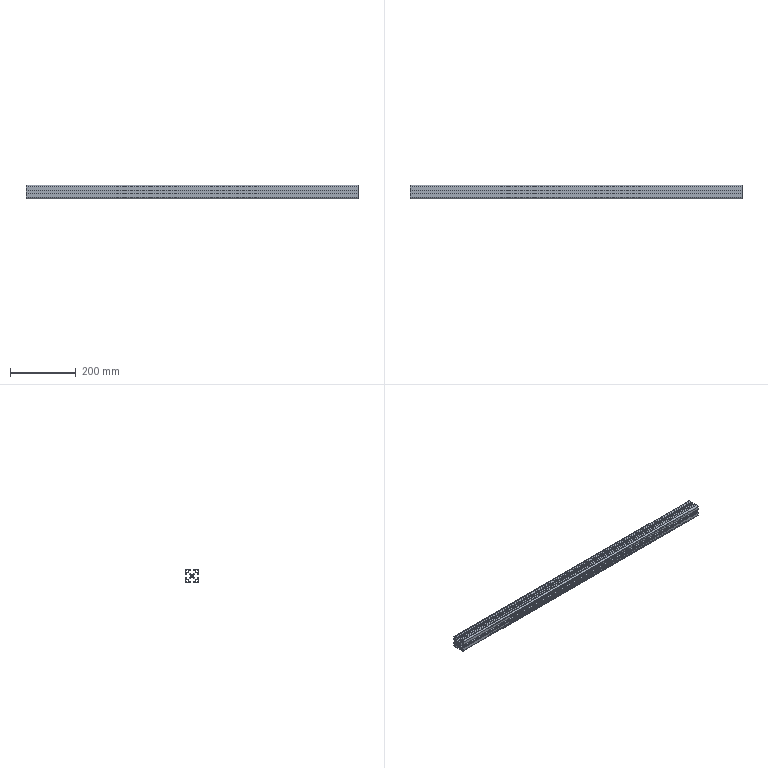Part | STEP file | MK-8-4040C-L-00 profile 4040C standard type 1010mm | 1 solid | 188 faces | box 1010 x 40 x 40 mm | volume 483031 mm3 | cylinder 94 | plane 94 | commonest cylinder face diameters 0.6 x30 2 x28 4 x16 0.4 x8 6 x4 9 x4